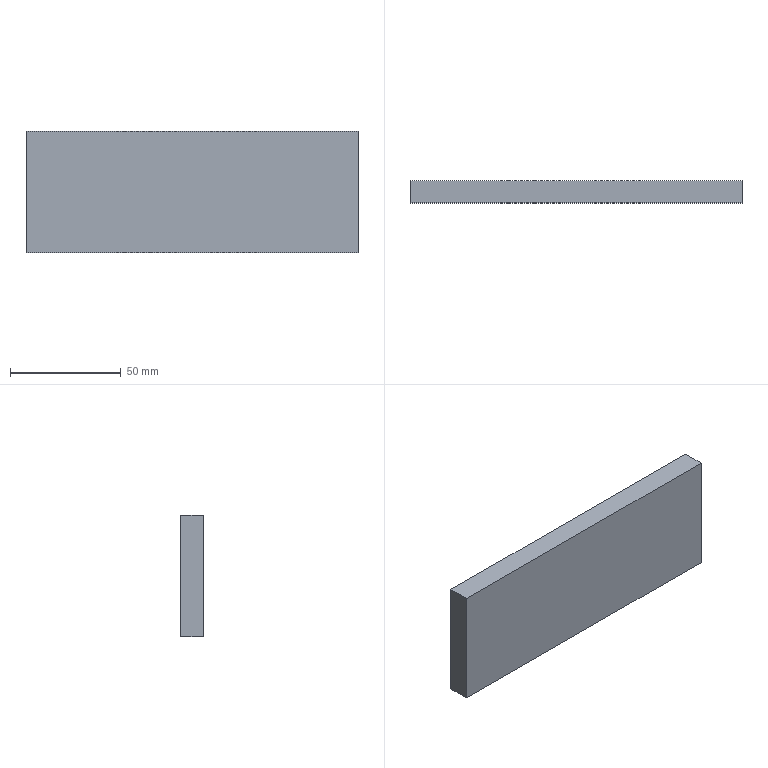Part | SolidWorks | features Extrusion 1 | 1 solid | 6 faces | box 150 x 10 x 55 mm | volume 82500 mm3 | plane 6
STEP:
#1=CARTESIAN_POINT('',(75.,-5.,0.));
#2=VERTEX_POINT('',#1);
#3=CARTESIAN_POINT('',(75.,5.,0.));
#4=VERTEX_POINT('',#3);
#5=CARTESIAN_POINT('',(75.,-5.,0.));
#6=DIRECTION('',(0.,1.,0.));
#7=VECTOR('',#6,1000.);
#8=LINE('',#5,#7);
#9=EDGE_CURVE('',#2,#4,#8,.T.);
#10=ORIENTED_EDGE('',*,*,#9,.T.);
#11=CARTESIAN_POINT('',(75.,5.,55.));
#12=VERTEX_POINT('',#11);
#13=CARTESIAN_POINT('',(75.,5.,55.));
#14=DIRECTION('',(0.,0.,-1.));
#15=VECTOR('',#14,1000.);
#16=LINE('',#13,#15);
#17=EDGE_CURVE('',#12,#4,#16,.T.);
#18=ORIENTED_EDGE('',*,*,#17,.F.);
#19=CARTESIAN_POINT('',(75.,-5.,55.));
#20=VERTEX_POINT('',#19);
#21=CARTESIAN_POINT('',(75.,-5.,55.));
#22=DIRECTION('',(0.,1.,0.));
#23=VECTOR('',#22,1000.);
#24=LINE('',#21,#23);
#25=EDGE_CURVE('',#20,#12,#24,.T.);
#26=ORIENTED_EDGE('',*,*,#25,.F.);
#27=CARTESIAN_POINT('',(75.,-5.,55.));
#28=DIRECTION('',(0.,0.,-1.));
#29=VECTOR('',#28,1000.);
#30=LINE('',#27,#29);
#31=EDGE_CURVE('',#20,#2,#30,.T.);
#32=ORIENTED_EDGE('',*,*,#31,.T.);
#33=EDGE_LOOP('',(#10,#18,#26,#32));
#34=FACE_OUTER_BOUND('',#33,.T.);
#35=CARTESIAN_POINT('',(75.,-5.,55.));
#36=DIRECTION('',(-1.,0.,0.));
#37=DIRECTION('',(0.,0.,1.));
#38=AXIS2_PLACEMENT_3D('',#35,#36,#37);
#39=PLANE('',#38);
#40=ADVANCED_FACE('',(#34),#39,.F.);
#41=CARTESIAN_POINT('',(-75.,5.,0.));
#42=VERTEX_POINT('',#41);
#43=CARTESIAN_POINT('',(-75.,5.,0.));
#44=DIRECTION('',(-1.,0.,0.));
#45=VECTOR('',#44,1000.);
#46=LINE('',#43,#45);
#47=EDGE_CURVE('',#4,#42,#46,.T.);
#48=ORIENTED_EDGE('',*,*,#47,.T.);
#49=CARTESIAN_POINT('',(-75.,5.,55.));
#50=VERTEX_POINT('',#49);
#51=CARTESIAN_POINT('',(-75.,5.,55.));
#52=DIRECTION('',(0.,0.,-1.));
#53=VECTOR('',#52,1000.);
#54=LINE('',#51,#53);
#55=EDGE_CURVE('',#50,#42,#54,.T.);
#56=ORIENTED_EDGE('',*,*,#55,.F.);
#57=CARTESIAN_POINT('',(-75.,5.,55.));
#58=DIRECTION('',(-1.,0.,0.));
#59=VECTOR('',#58,1000.);
#60=LINE('',#57,#59);
#61=EDGE_CURVE('',#12,#50,#60,.T.);
#62=ORIENTED_EDGE('',*,*,#61,.F.);
#63=ORIENTED_EDGE('',*,*,#17,.T.);
#64=EDGE_LOOP('',(#48,#56,#62,#63));
#65=FACE_OUTER_BOUND('',#64,.T.);
#66=CARTESIAN_POINT('',(-75.,5.,55.));
#67=DIRECTION('',(0.,-1.,0.));
#68=DIRECTION('',(0.,0.,-1.));
#69=AXIS2_PLACEMENT_3D('',#66,#67,#68);
#70=PLANE('',#69);
#71=ADVANCED_FACE('',(#65),#70,.F.);
#72=CARTESIAN_POINT('',(-75.,-5.,0.));
#73=VERTEX_POINT('',#72);
#74=CARTESIAN_POINT('',(-75.,-5.,0.));
#75=DIRECTION('',(0.,-1.,0.));
#76=VECTOR('',#75,1000.);
#77=LINE('',#74,#76);
#78=EDGE_CURVE('',#42,#73,#77,.T.);
#79=ORIENTED_EDGE('',*,*,#78,.T.);
#80=CARTESIAN_POINT('',(-75.,-5.,55.));
#81=VERTEX_POINT('',#80);
#82=CARTESIAN_POINT('',(-75.,-5.,55.));
#83=DIRECTION('',(0.,0.,-1.));
#84=VECTOR('',#83,1000.);
#85=LINE('',#82,#84);
#86=EDGE_CURVE('',#81,#73,#85,.T.);
#87=ORIENTED_EDGE('',*,*,#86,.F.);
#88=CARTESIAN_POINT('',(-75.,-5.,55.));
#89=DIRECTION('',(0.,-1.,0.));
#90=VECTOR('',#89,1000.);
#91=LINE('',#88,#90);
#92=EDGE_CURVE('',#50,#81,#91,.T.);
#93=ORIENTED_EDGE('',*,*,#92,.F.);
#94=ORIENTED_EDGE('',*,*,#55,.T.);
#95=EDGE_LOOP('',(#79,#87,#93,#94));
#96=FACE_OUTER_BOUND('',#95,.T.);
#97=CARTESIAN_POINT('',(-75.,-5.,55.));
#98=DIRECTION('',(1.,0.,0.));
#99=DIRECTION('',(0.,0.,-1.));
#100=AXIS2_PLACEMENT_3D('',#97,#98,#99);
#101=PLANE('',#100);
#102=ADVANCED_FACE('',(#96),#101,.F.);
#103=CARTESIAN_POINT('',(-75.,-5.,0.));
#104=DIRECTION('',(1.,0.,0.));
#105=VECTOR('',#104,1000.);
#106=LINE('',#103,#105);
#107=EDGE_CURVE('',#73,#2,#106,.T.);
#108=ORIENTED_EDGE('',*,*,#107,.T.);
#109=ORIENTED_EDGE('',*,*,#31,.F.);
#110=CARTESIAN_POINT('',(-75.,-5.,55.));
#111=DIRECTION('',(1.,0.,0.));
#112=VECTOR('',#111,1000.);
#113=LINE('',#110,#112);
#114=EDGE_CURVE('',#81,#20,#113,.T.);
#115=ORIENTED_EDGE('',*,*,#114,.F.);
#116=ORIENTED_EDGE('',*,*,#86,.T.);
#117=EDGE_LOOP('',(#108,#109,#115,#116));
#118=FACE_OUTER_BOUND('',#117,.T.);
#119=CARTESIAN_POINT('',(-75.,-5.,55.));
#120=DIRECTION('',(0.,1.,0.));
#121=DIRECTION('',(0.,0.,1.));
#122=AXIS2_PLACEMENT_3D('',#119,#120,#121);
#123=PLANE('',#122);
#124=ADVANCED_FACE('',(#118),#123,.F.);
#125=ORIENTED_EDGE('',*,*,#25,.T.);
#126=ORIENTED_EDGE('',*,*,#61,.T.);
#127=ORIENTED_EDGE('',*,*,#92,.T.);
#128=ORIENTED_EDGE('',*,*,#114,.T.);
#129=EDGE_LOOP('',(#125,#126,#127,#128));
#130=FACE_OUTER_BOUND('',#129,.T.);
#131=CARTESIAN_POINT('',(0.,0.,55.));
#132=DIRECTION('',(0.,0.,-1.));
#133=DIRECTION('',(-1.,0.,0.));
#134=AXIS2_PLACEMENT_3D('',#131,#132,#133);
#135=PLANE('',#134);
#136=ADVANCED_FACE('',(#130),#135,.F.);
#137=ORIENTED_EDGE('',*,*,#9,.F.);
#138=ORIENTED_EDGE('',*,*,#107,.F.);
#139=ORIENTED_EDGE('',*,*,#78,.F.);
#140=ORIENTED_EDGE('',*,*,#47,.F.);
#141=EDGE_LOOP('',(#137,#138,#139,#140));
#142=FACE_OUTER_BOUND('',#141,.T.);
#143=CARTESIAN_POINT('',(0.,0.,0.));
#144=DIRECTION('',(0.,0.,-1.));
#145=DIRECTION('',(-1.,0.,0.));
#146=AXIS2_PLACEMENT_3D('',#143,#144,#145);
#147=PLANE('',#146);
#148=ADVANCED_FACE('',(#142),#147,.T.);
#149=CLOSED_SHELL('',(#40,#71,#102,#124,#136,#148));
#150=MANIFOLD_SOLID_BREP('',#149);
#151=CARTESIAN_POINT('',(0.,0.,0.));
#152=DIRECTION('',(0.,0.,1.));
#153=DIRECTION('',(1.,0.,0.));
#154=AXIS2_PLACEMENT_3D('',#151,#152,#153);
#155=(LENGTH_UNIT()NAMED_UNIT(*)SI_UNIT(.MILLI.,.METRE.));
#156=UNCERTAINTY_MEASURE_WITH_UNIT(LENGTH_MEASURE(0.00001),#155,'','');
#157=(NAMED_UNIT(*)PLANE_ANGLE_UNIT()SI_UNIT($,.RADIAN.));
#158=(NAMED_UNIT(*)SI_UNIT($,.STERADIAN.)SOLID_ANGLE_UNIT());
#159=(GEOMETRIC_REPRESENTATION_CONTEXT(3)GLOBAL_UNCERTAINTY_ASSIGNED_CONTEXT((#156))GLOBAL_UNIT_ASSIGNED_CONTEXT((#155,#157,#158))REPRESENTATION_CONTEXT('',''));
#160=ADVANCED_BREP_SHAPE_REPRESENTATION('',(#150,#154),#159);